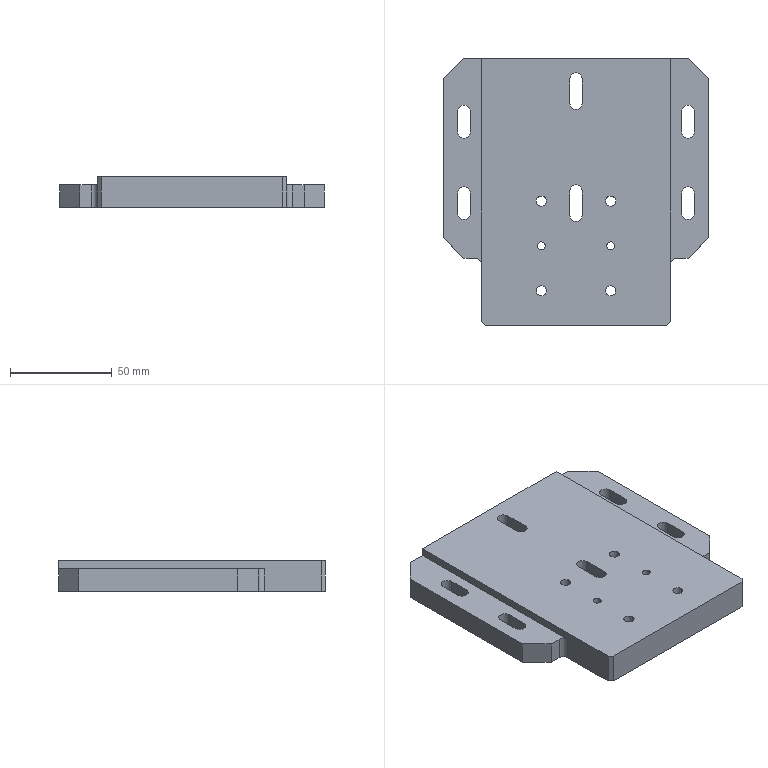Part | 1 solid | 56 faces | box 130 x 131 x 15 mm | volume 211794 mm3 | plane 30 | cylinder 26 | commonest cylinder face diameters 5 x8 6.2 x8 6 x6 4 x4